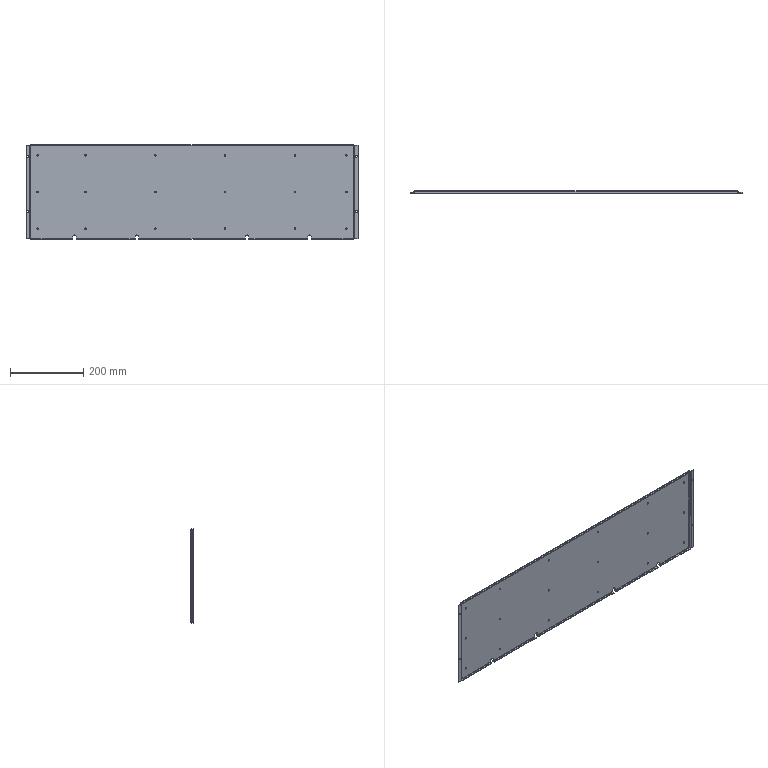Part | STEP file | 1 solid | 138 faces | box 904 x 7 x 258 mm | volume 482267 mm3 | cylinder 80 | plane 58 | commonest cylinder face diameters 4.2 x44 10 x16 2 x10 6 x10